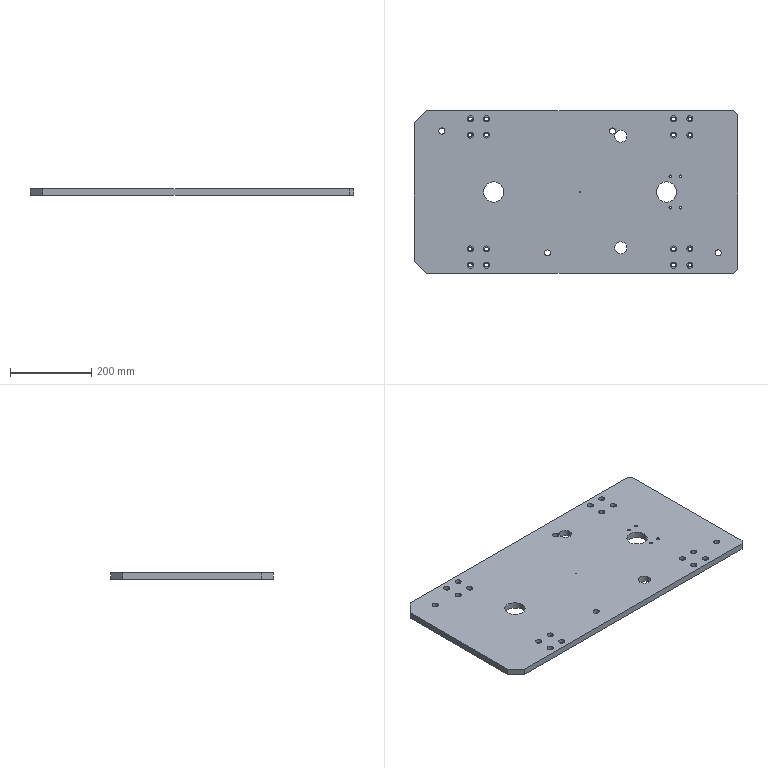Part | SolidWorks | features BaseBody 1 | 1 solid | 116 faces | box 795 x 400 x 16 mm | volume 4940292 mm3 | cylinder 90 | plane 26 | commonest cylinder face diameters 15 x40 9 x32 6.8 x8 30 x4 50 x4 2 x2